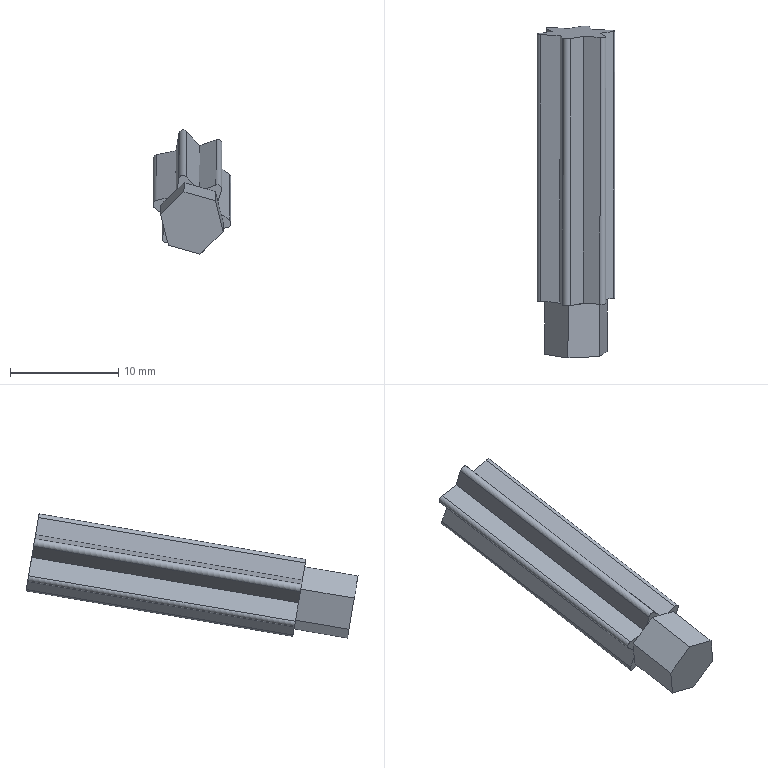Part | STEP file | Dodanie-wyci_gni_cie2_4 | 1 solid | 40 faces | box 7.193 x 30.668 x 11.467 mm | volume 797.649 mm3 | plane 32 | cylinder 8 | commonest cylinder face diameters 0.798 x8